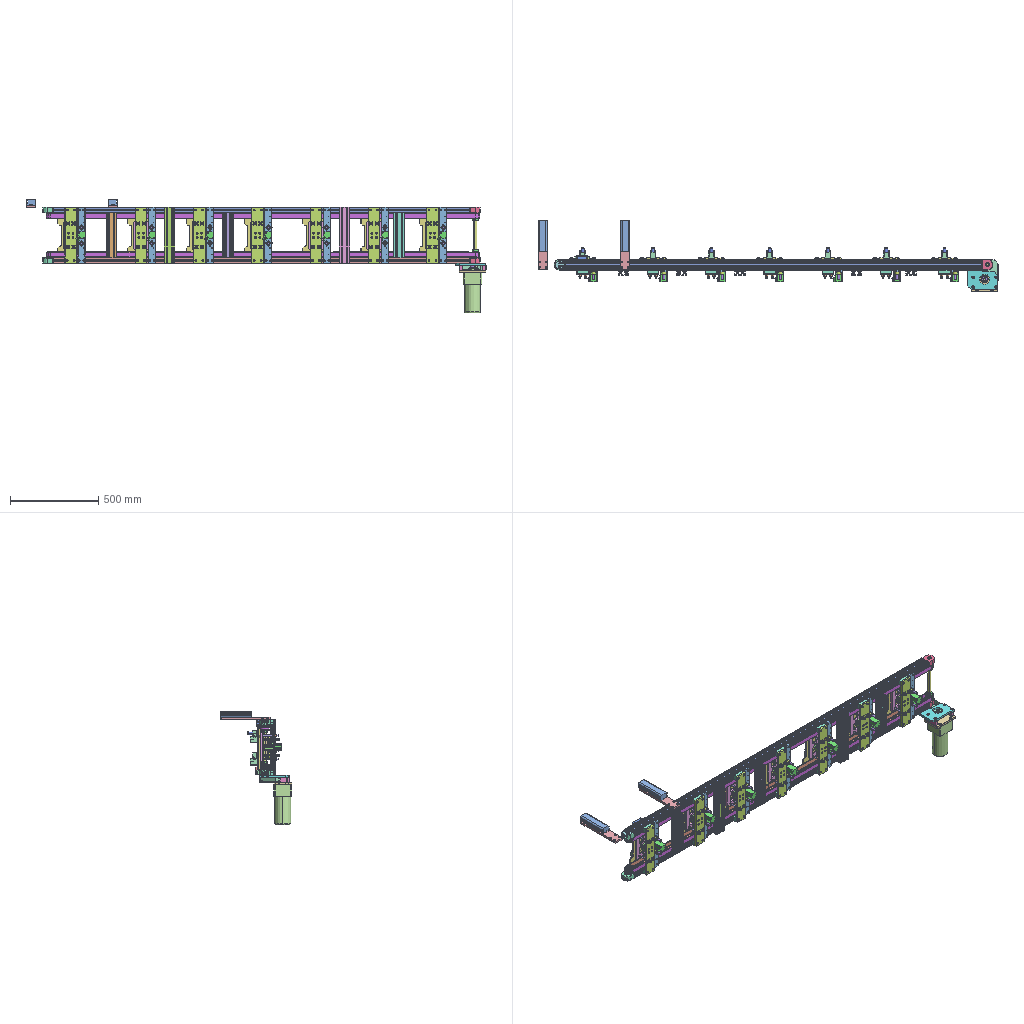Assembly | STEP file | 51 different items | 323 placed | box 2604 x 407 x 644 mm
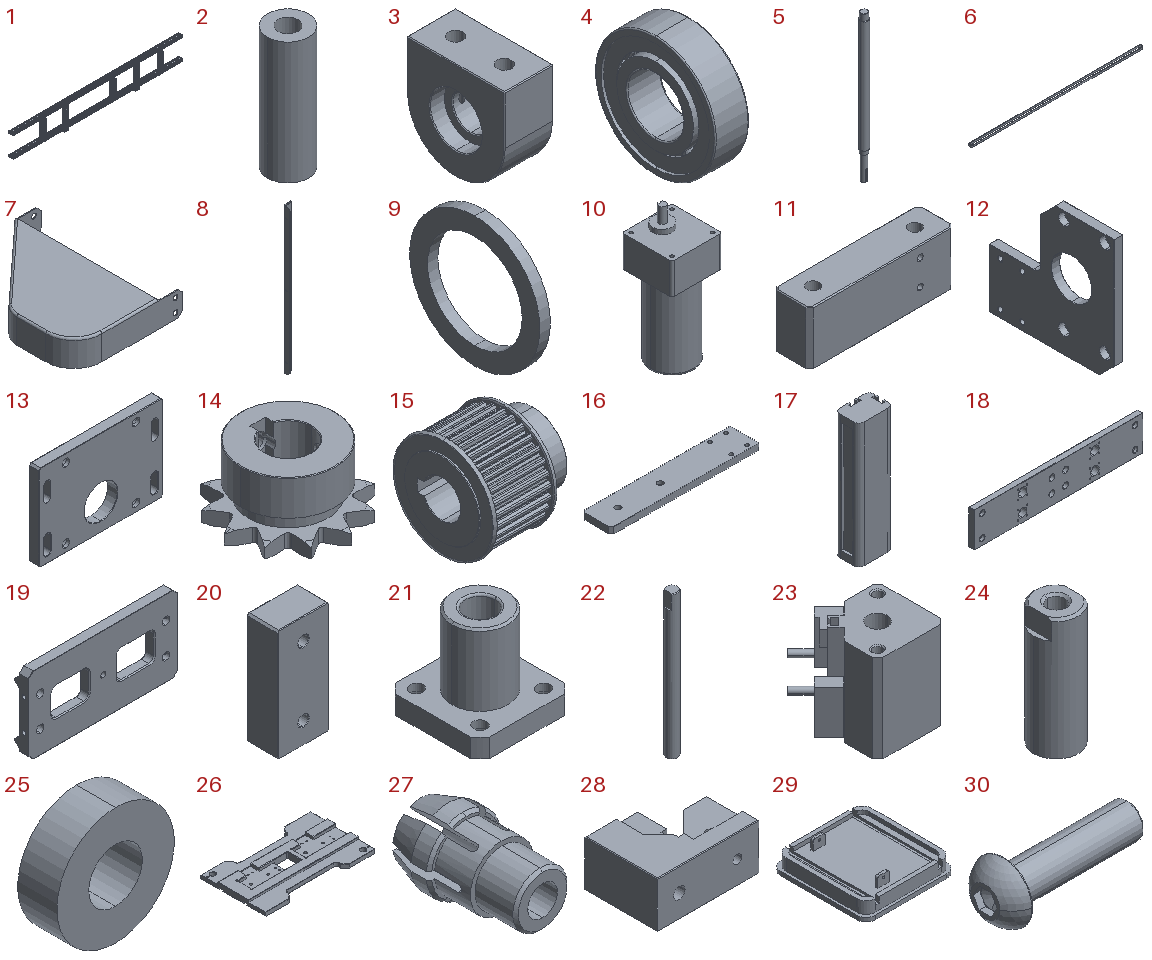Parts list (item | name | quantity | parent item | size | volume):
1 | welding conveyor bracket 01_Default <Machining> | x1 | - | 2360 x 90 x 316 mm | 3445395 mm3
2 | PN_0027 threaded bushing_Default | x8 | - | 10 x 10 x 30 mm | 1767 mm3
3 | PN_0009 hoist driving shaft fixing plate_Default | x2 | - | 30 x 60 x 60 mm | 72459 mm3
4 | GB/T 276-94 deep groove ball bearing 6002-2Z | x2 | - | 9 x 32 x 32 mm | 3545 mm3
5 | PN_0011 drive shaft_Default | x1 | - | 18 x 18 x 335 mm | 73475 mm3
6 | welding conveyor belt_Default | x2 | - | 2454 x 51.95 x 25 mm | 495464 mm3
7 | PN_0003 stopper | x1 | - | 117 x 152.64 x 28 mm | 18137 mm3
8 | PN_0005 long bracket plate_Default | x6 | - | 35 x 30 x 774.978 mm | 94609 mm3
9 | PN_0010 positioning ring_Default | x2 | - | 2 x 25 x 25 mm | 461.437 mm3
10 | Taibang reversible motor 90W_Default | x1 | in motor assembly_Default | 104 x 104 x 269 mm | 1739193 mm3
11 | PN_0002 motor pillar_Default | x2 | in motor assembly_Default | 80 x 20 x 30 mm | 45190 mm3
12 | PN_0001 motor fixing plate_Default | x1 | in motor assembly_Default | 12 x 170 x 170 mm | 228176 mm3
13 | 180W motor mounting plate_Default | x1 | in motor assembly_Default | 150 x 12 x 104 mm | 156125 mm3
14 | SP35B12_N_15_SP35B12-N-15 | x1 | in motor assembly_Default | 41 x 41 x 20 mm | 10343 mm3
15 | PN_0012 T5 synchronous pulley 30 teeth 1 | x2 | - | 44 x 49 x 49 mm | 49129 mm3
16 | PN_0004 light curtain mounting bracket plate_Default | x2 | - | 280 x 55 x 12 mm | 179701 mm3
17 | light curtain sensor_Default | x2 | - | 50 x 35 x 180 mm | 266071 mm3
18 | lifting air cylinder fixing support seat 01 | x7 | in fixture lifting mechanism assembly drawing | 316 x 10 x 65 mm | 191391 mm3
19 | lifting air cylinder fixing support seat 02 | x7 | in fixture lifting mechanism assembly drawing | 160 x 15 x 82 mm | 115095 mm3
20 | lifting air cylinder fixing support seat 03 | x14 | in fixture lifting mechanism assembly drawing | 30 x 18 x 65 mm | 34026 mm3
21 | linear bearing LMK8UU_Default | x28 | in fixture lifting mechanism assembly drawing | 25 x 25 x 24 mm | 4786 mm3
22 | positioning guide rod | x28 | in fixture lifting mechanism assembly drawing | 8 x 8 x 100 mm | 4985 mm3
23 | CDQ2A20_15D_F7NV0 | x7 | in fixture lifting mechanism assembly drawing | 48.335 x 48.335 x 46.5 mm | 53480 mm3
24 | CDQ2A20_15D_1_F7NV0 | x7 | in fixture lifting mechanism assembly drawing | 10 x 10 x 27.5 mm | 2020 mm3
25 | PN_0026 lifting mechanism plate_Default | x7 | in fixture lifting mechanism assembly drawing | 12 x 4 x 12 mm | 357.356 mm3
26 | base hole locating fixture plate | x7 | in experiment use | 255 x 150 x 14 mm | 299894 mm3
27 | 8mm elastic locating pin | x14 | in experiment use | 8.161 x 13.5 x 8.2 mm | 235.099 mm3
28 | product fixture | x28 | in product fixture_Default, experiment use | 70 x 50 x 32 mm | 81575 mm3
29 | product_Default | x12 | in product fixture_Default | 23 x 24 x 5.6 mm | 1586 mm3
30 | socket button head screw_iso_PreviewCfg | x7 | in experiment use | 68.8 x 28 x 28 mm | 15482 mm3
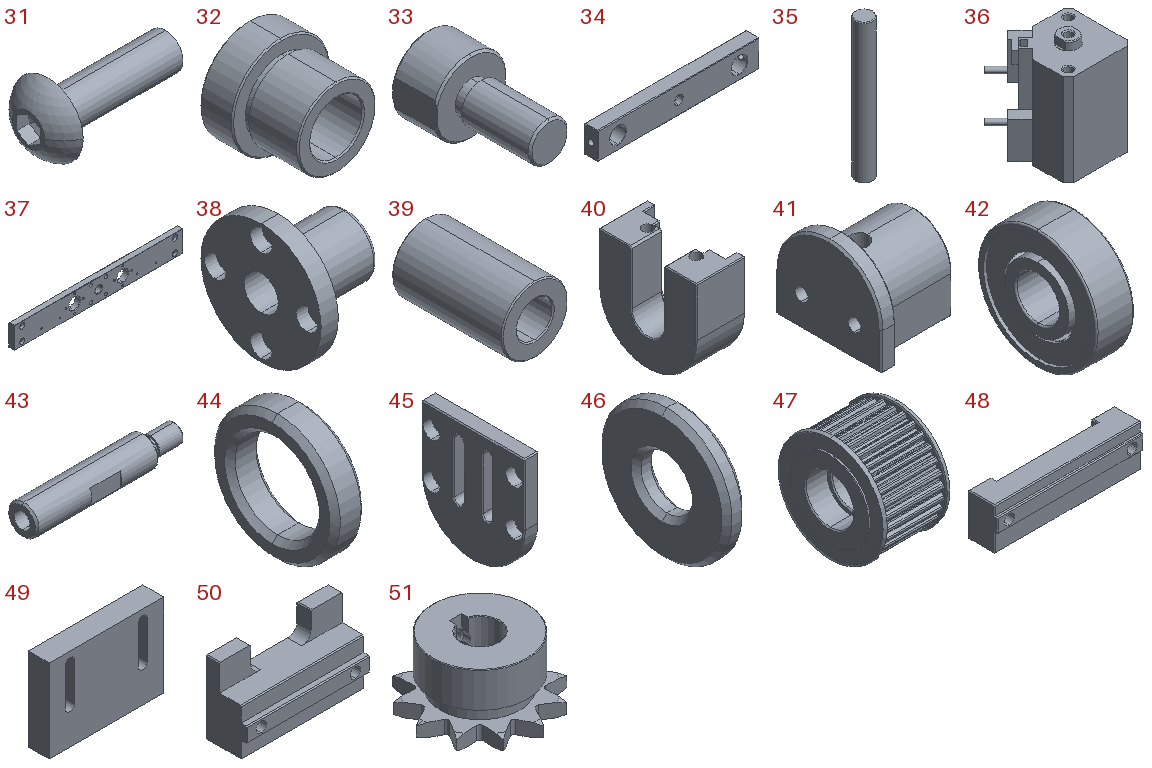31 | hexagon socket button head screws gb_PreviewCfg | x7 | in experiment use | 23.3 x 12 x 12 mm | 775.96 mm3
32 | PN_0020 side positioning guide sleeve_Default | x14 | in experiment use | 15 x 13.5 x 15 mm | 1145 mm3
33 | PN_0021 fixture block | x14 | in experiment use | 7 x 12.5 x 7.5 mm | 290.271 mm3
34 | PN_0023 lifting connecting plate_Default | x7 | in universal test stopper 12_Default | 120 x 10 x 20 mm | 20677 mm3
35 | PN_0024 test guide rod_Default | x14 | in universal test stopper 12_Default | 12 x 12 x 95 mm | 10735 mm3
36 | A_CDQ2A25-25D-F7NV012_Default | x7 | in universal test stopper 12_Default | 52.598 x 52.598 x 62.5 mm | 85379 mm3
37 | PN_0022 stopper air cylinder fixing seat | x7 | in universal test stopper 12_Default | 316 x 10 x 40 mm | 112914 mm3
38 | LHFR122_Default | x14 | in universal test stopper 12_Default | 30 x 42 x 42 mm | 12352 mm3
39 | PN_0025 lifting air cylinder extension rod_Default | x7 | in universal test stopper 12_Default | 12 x 20 x 12 mm | 1596 mm3
40 | PN_0013 driven wheel mounting plate_Default | x2 | in driven wheel assembly_Default | 30 x 60 x 60 mm | 50936 mm3
41 | PN_0014 driven wheel fixing block_Default | x2 | in driven wheel assembly_Default | 23 x 28 x 24 mm | 8364 mm3
42 | GB/T 276-94 deep groove ball bearing 608-2Z | x4 | in driven wheel assembly_Default | 7 x 22 x 22 mm | 1460 mm3
43 | PN_0016 fixed shaft_Default | x2 | in driven wheel assembly_Default | 40.5 x 8 x 8 mm | 1575 mm3
44 | PN_0017 driven wheel limiting round block_Default | x2 | in driven wheel assembly_Default | 3 x 12 x 12 mm | 168.916 mm3
45 | PN_0015 press block_Default | x2 | in driven wheel assembly_Default | 7 x 50 x 55 mm | 14443 mm3
46 | PN_0018 driven wheel fixing round block_Default | x2 | in driven wheel assembly_Default | 2 x 13 x 13 mm | 208.696 mm3
47 | PN_0019 T5 synchronous pulley 30 teeth 2 | x2 | in driven wheel assembly_Default | 32 x 49 x 49 mm | 40684 mm3
48 | PN_0006 fixture positioning -V-shape edge 2-2_Default | x1 | in press product locating assembly_Default | 80 x 16 x 23 mm | 22056 mm3
49 | PN_0007 fixture positioning -V-shape edge 1-2_Default | x1 | in press product locating assembly_Default | 55 x 10 x 40 mm | 20062 mm3
50 | PN_0008 fixture positioning plate 156 stations_Default | x1 | - | 65 x 22 x 39 mm | 33983 mm3
51 | SP35B12_N_12_SP35B12-N-12 | x1 | - | 41 x 41 x 20 mm | 11740 mm3
Placements (level | parent | child | x y z in mm | rotation matrix by rows):
1 | subassembly 2 | welding conveyor bracket 01_Default <Machining> | -0.0 -0.0 -0.0 | -1 0 0 0 1 0 0 0 -1
1 | subassembly 2 | PN_0027 threaded bushing_Default | 1150.0 15.0 -143.0 | 0 0 1 0 1 0 -1 0 0
1 | subassembly 2 | PN_0027 threaded bushing_Default | 1150.0 -15.0 -143.0 | 0 0 1 0.9242 -0.3818 0 0.3818 0.9242 0
1 | subassembly 2 | PN_0027 threaded bushing_Default | -1180.0 -15.0 143.0 | 0 0 1 0.007845 1 0 -1 0.007845 0
1 | subassembly 2 | PN_0027 threaded bushing_Default | -1180.0 15.0 143.0 | 0 0 1 0 1 0 -1 0 0
1 | subassembly 2 | PN_0027 threaded bushing_Default | -1180.0 15.0 -143.0 | 0 0 1 0 1 0 -1 0 0
1 | subassembly 2 | PN_0027 threaded bushing_Default | -1180.0 -15.0 -143.0 | 0 0 1 0 1 0 -1 0 0
1 | subassembly 2 | PN_0027 threaded bushing_Default | 1150.0 -15.0 143.0 | 0 0 1 0 1 0 -1 0 0
1 | subassembly 2 | PN_0027 threaded bushing_Default | 1150.0 15.0 143.0 | 0 0 1 0 1 0 -1 0 0
1 | subassembly 2 | PN_0009 hoist driving shaft fixing plate_Default | 1195.0 0.0 -128.0 | 0 0 -1 0 -1 0 -1 0 0
1 | subassembly 2 | PN_0009 hoist driving shaft fixing plate_Default | 1195.0 -0.0 128.0 | 0 0 -1 0 1 0 1 0 0
1 | subassembly 2 | GB/T 276-94 deep groove ball bearing 6002-2Z | 1210.0 0.0 132.5 | 0 0 -1 0 1 0 1 0 0
1 | subassembly 2 | GB/T 276-94 deep groove ball bearing 6002-2Z | 1210.0 0.0 -132.5 | 0 0 -1 0 1 0 1 0 0
1 | subassembly 2 | PN_0011 drive shaft_Default | 1210.0 -0.0 142.0 | 0.4483 -0.8939 0 0.8939 0.4483 0 0 0 1
1 | subassembly 2 | welding conveyor belt_Default | 1210.0 -0.0 -97.5 | -1 0 0 0 -1 0 0 0 1
1 | subassembly 2 | welding conveyor belt_Default | 1210.0 -0.0 122.5 | -1 0 0 0 -1 0 0 0 1
1 | subassembly 2 | PN_0003 stopper | 1241.0 -0.0 -170.0 | 0 -1 0 -1 0 0 0 0 -1
1 | subassembly 2 | PN_0005 long bracket plate_Default | -782.5 21.975 -110.5 | 0 0 -1 0 1 0 1 0 0
1 | subassembly 2 | PN_0010 positioning ring_Default | 1210.0 -0.0 -126.0 | 0 -0.5087 -0.8609 0 -0.8609 0.5087 -1 0 0
1 | subassembly 2 | PN_0010 positioning ring_Default | 1210.0 -0.0 128.0 | 0 0 1 0 1 0 -1 0 -0
1 | subassembly 2 | motor assembly_Default | 1161.778 -91.728 -283.549 | 1 0 0 0 1 0 0 0 1
2 | motor assembly_Default | Taibang reversible motor 90W_Default | 33.222 -10.273 6.549 | 1 0 0 0 1 0 0 0 1
2 | motor assembly_Default | PN_0002 motor pillar_Default | 98.222 -8.273 98.549 | 0 -1 0 1 0 0 0 0 1
2 | motor assembly_Default | PN_0002 motor pillar_Default | -31.778 -8.273 98.549 | 0 -1 0 1 0 0 0 0 1
2 | motor assembly_Default | PN_0001 motor fixing plate_Default | 23.222 36.727 125.549 | 0 0 1 0 1 0 -1 0 0
2 | motor assembly_Default | 180W motor mounting plate_Default | 33.222 -10.273 71.549 | 1 0 0 0 0 -1 0 1 0
2 | motor assembly_Default | SP35B12_N_15_SP35B12-N-15 | 33.222 9.727 93.549 | 1 0 0 0 1 0 0 0 1
1 | subassembly 2 | PN_0012 T5 synchronous pulley 30 teeth 1 | 1210.0 -0.0 -126.0 | 0 -0.8939 -0.4483 0 0.4483 -0.8939 1 0 -0
1 | subassembly 2 | PN_0012 T5 synchronous pulley 30 teeth 1 | 1210.0 -0.0 126.0 | 0 -0.8939 0.4483 0 0.4483 0.8939 -1 0 0
1 | subassembly 2 | PN_0004 light curtain mounting bracket plate_Default | -1305.745 110.0 170.0 | 0 -1 0 -1 0 0 0 0 -1
1 | subassembly 2 | light curtain sensor_Default | -1305.745 252.622 187.5 | -1 0 0 0 0 -1 0 -1 0
1 | subassembly 2 | PN_0004 light curtain mounting bracket plate_Default | -840.5 110.0 170.0 | 0 -1 0 -1 0 0 0 0 -1
1 | subassembly 2 | light curtain sensor_Default | -840.5 72.622 187.5 | 1 0 0 0 0 1 0 -1 -0
1 | subassembly 2 | PN_0005 long bracket plate_Default | 2.5 21.975 -110.5 | 0 0 -1 0 1 0 1 0 0
1 | subassembly 2 | PN_0005 long bracket plate_Default | 787.5 21.975 -110.5 | 0 0 -1 0 1 0 1 0 0
1 | subassembly 2 | PN_0005 long bracket plate_Default | 787.5 21.975 110.5 | 0 0 1 0 1 0 -1 0 0
1 | subassembly 2 | PN_0005 long bracket plate_Default | 2.5 21.975 110.5 | 0 0 1 0 1 0 -1 0 0
1 | subassembly 2 | PN_0005 long bracket plate_Default | -782.5 21.975 110.5 | 0 0 1 0 1 0 -1 0 0
1 | subassembly 2 | fixture lifting mechanism assembly drawing | -1080.0 -58.0 -0.0 | 0 0 1 0 1 0 -1 0 0
2 | fixture lifting mechanism assembly drawing | lifting air cylinder fixing support seat 01 | -0.0 -0.0 -0.0 | 1 0 0 0 1 0 0 0 1
2 | fixture lifting mechanism assembly drawing | lifting air cylinder fixing support seat 02 | -0.0 77.202 -0.0 | -1 0 0 0 1 0 0 0 -1
2 | fixture lifting mechanism assembly drawing | lifting air cylinder fixing support seat 03 | -143.0 10.0 -0.0 | 1 0 0 0 1 0 0 0 1
2 | fixture lifting mechanism assembly drawing | lifting air cylinder fixing support seat 03 | 143.0 10.0 -0.0 | -1 0 0 0 1 0 0 0 -1
2 | fixture lifting mechanism assembly drawing | linear bearing LMK8UU_Default | -67.5 15.0 -16.5 | 1 0 0 0 0 -1 0 1 -0
2 | fixture lifting mechanism assembly drawing | linear bearing LMK8UU_Default | -67.5 15.0 16.5 | 1 0 0 0 0 -1 0 1 -0
2 | fixture lifting mechanism assembly drawing | linear bearing LMK8UU_Default | 67.5 15.0 16.5 | 1 0 0 0 0 -1 0 1 -0
2 | fixture lifting mechanism assembly drawing | linear bearing LMK8UU_Default | 67.5 15.0 -16.5 | 1 0 0 0 0 -1 0 1 -0
2 | fixture lifting mechanism assembly drawing | positioning guide rod | -67.5 32.202 16.5 | 1 0 0 0 0 1 0 -1 -0
2 | fixture lifting mechanism assembly drawing | positioning guide rod | 67.5 32.202 16.5 | -1 0 0 0 0 1 0 1 0
2 | fixture lifting mechanism assembly drawing | positioning guide rod | -67.5 32.202 -16.5 | 1 0 0 0 0 1 0 -1 -0
2 | fixture lifting mechanism assembly drawing | positioning guide rod | 67.5 32.202 -16.5 | -1 0 0 0 0 1 0 1 0
2 | fixture lifting mechanism assembly drawing | CDQ2A20_15D_F7NV0 | -0.0 56.5 0.0 | 1 0 0 0 0 1 0 -1 0
2 | fixture lifting mechanism assembly drawing | CDQ2A20_15D_1_F7NV0 | -0.0 63.702 0.0 | -0.9915 0.13 0 0 0 1 0.13 0.9915 0
2 | fixture lifting mechanism assembly drawing | PN_0026 lifting mechanism plate_Default | -0.0 68.202 0.0 | 1 0 0 0 1 0 0 0 1
1 | subassembly 2 | fixture lifting mechanism assembly drawing | -682.044 -58.0 -0.0 | 0 0 1 0 1 0 -1 0 0
2 | fixture lifting mechanism assembly drawing | lifting air cylinder fixing support seat 01 | -0.0 -0.0 -0.0 | 1 0 0 0 1 0 0 0 1
2 | fixture lifting mechanism assembly drawing | lifting air cylinder fixing support seat 02 | -0.0 77.202 -0.0 | -1 0 0 0 1 0 0 0 -1
2 | fixture lifting mechanism assembly drawing | lifting air cylinder fixing support seat 03 | -143.0 10.0 -0.0 | 1 0 0 0 1 0 0 0 1
2 | fixture lifting mechanism assembly drawing | lifting air cylinder fixing support seat 03 | 143.0 10.0 -0.0 | -1 0 0 0 1 0 0 0 -1
2 | fixture lifting mechanism assembly drawing | linear bearing LMK8UU_Default | -67.5 15.0 -16.5 | 1 0 0 0 0 -1 0 1 -0
2 | fixture lifting mechanism assembly drawing | linear bearing LMK8UU_Default | -67.5 15.0 16.5 | 1 0 0 0 0 -1 0 1 -0
2 | fixture lifting mechanism assembly drawing | linear bearing LMK8UU_Default | 67.5 15.0 16.5 | 1 0 0 0 0 -1 0 1 -0
2 | fixture lifting mechanism assembly drawing | linear bearing LMK8UU_Default | 67.5 15.0 -16.5 | 1 0 0 0 0 -1 0 1 -0
2 | fixture lifting mechanism assembly drawing | positioning guide rod | -67.5 32.202 16.5 | 1 0 0 0 0 1 0 -1 -0
2 | fixture lifting mechanism assembly drawing | positioning guide rod | 67.5 32.202 16.5 | -1 0 0 0 0 1 0 1 0
2 | fixture lifting mechanism assembly drawing | positioning guide rod | -67.5 32.202 -16.5 | 1 0 0 0 0 1 0 -1 -0
2 | fixture lifting mechanism assembly drawing | positioning guide rod | 67.5 32.202 -16.5 | -1 0 0 0 0 1 0 1 0
2 | fixture lifting mechanism assembly drawing | CDQ2A20_15D_F7NV0 | -0.0 56.5 0.0 | 1 0 0 0 0 1 0 -1 0
2 | fixture lifting mechanism assembly drawing | CDQ2A20_15D_1_F7NV0 | -0.0 63.702 0.0 | -0.9915 0.13 0 0 0 1 0.13 0.9915 0
2 | fixture lifting mechanism assembly drawing | PN_0026 lifting mechanism plate_Default | -0.0 68.202 0.0 | 1 0 0 0 1 0 0 0 1
1 | subassembly 2 | experiment use | -1087.0 25.975 6.807 | 0 0 -1 0 1 0 1 0 -0
2 | experiment use | base hole locating fixture plate | -9.307 -0.0 -7.0 | 1 0 0 0 0 1 0 -1 -0
2 | experiment use | 8mm elastic locating pin | -92.307 2.5 -7.0 | 1 0 -0.006215 0 1 0 0.006215 0 1
2 | experiment use | 8mm elastic locating pin | 33.693 2.5 -7.0 | 1 0 0 0 1 0 0 0 1
2 | experiment use | product fixture_Default | -90.399 12.134 -29.041 | 1 0 0 0 1 0 0 0 1
3 | product fixture_Default | product fixture | -16.908 -5.134 22.041 | 1 0 0 0 1 0 0 0 1
3 | product fixture_Default | product_Default | 27.224 21.108 22.041 | -0.7071 0 -0.7071 -0.7071 0 0.7071 0 1 -0
2 | experiment use | product fixture_Default | 35.601 12.134 -29.041 | 1 0 0 0 1 0 0 0 1
3 | product fixture_Default | product fixture | -16.908 -5.134 22.041 | 1 0 0 0 1 0 0 0 1
3 | product fixture_Default | product_Default | 27.224 21.108 22.041 | -0.7071 0 -0.7071 -0.7071 0 0.7071 0 1 -0
2 | experiment use | socket button head screw_iso_PreviewCfg | 73.693 0.35 -7.0 | 0 -1 0 1 0 0 0 0 1
2 | experiment use | hexagon socket button head screws gb_PreviewCfg | 33.693 -0.8 -7.0 | 0 -1 0 1 0 0 0 0 1
2 | experiment use | product fixture | -107.307 7.0 -7.0 | 1 0 0 0 1 0 0 0 1
2 | experiment use | product fixture | 18.693 7.0 -7.0 | 1 0 0 0 1 0 0 0 1
2 | experiment use | PN_0020 side positioning guide sleeve_Default | 104.693 0.5 55.75 | -0.6791 0 0.734 0 1 0 -0.734 0 -0.6791
2 | experiment use | PN_0020 side positioning guide sleeve_Default | -118.307 0.5 -69.75 | 0.6258 0 -0.78 0 1 0 0.78 0 0.6258
2 | experiment use | PN_0021 fixture block | 116.193 9.0 55.75 | 1 0 0 0 1 0 0 0 1
2 | experiment use | PN_0021 fixture block | -129.807 9.0 -69.75 | 1 0 0 0 1 0 0 0 1
1 | subassembly 2 | experiment use | -689.044 25.975 6.807 | 0 0 -1 0 1 0 1 0 -0
2 | experiment use | base hole locating fixture plate | -9.307 -0.0 -7.0 | 1 0 0 0 0 1 0 -1 -0
2 | experiment use | 8mm elastic locating pin | -92.307 2.5 -7.0 | 1 0 -0.006215 0 1 0 0.006215 0 1
2 | experiment use | 8mm elastic locating pin | 33.693 2.5 -7.0 | 1 0 0 0 1 0 0 0 1
2 | experiment use | product fixture_Default | -90.399 12.134 -29.041 | 1 0 0 0 1 0 0 0 1
3 | product fixture_Default | product fixture | -16.908 -5.134 22.041 | 1 0 0 0 1 0 0 0 1
3 | product fixture_Default | product_Default | 27.224 21.108 22.041 | -0.7071 0 -0.7071 -0.7071 0 0.7071 0 1 -0
2 | experiment use | product fixture_Default | 35.601 12.134 -29.041 | 1 0 0 0 1 0 0 0 1
3 | product fixture_Default | product fixture | -16.908 -5.134 22.041 | 1 0 0 0 1 0 0 0 1
3 | product fixture_Default | product_Default | 27.224 21.108 22.041 | -0.7071 0 -0.7071 -0.7071 0 0.7071 0 1 -0
2 | experiment use | socket button head screw_iso_PreviewCfg | 73.693 0.35 -7.0 | 0 -1 0 1 0 0 0 0 1
2 | experiment use | hexagon socket button head screws gb_PreviewCfg | 33.693 -0.8 -7.0 | 0 -1 0 1 0 0 0 0 1
2 | experiment use | product fixture | -107.307 7.0 -7.0 | 1 0 0 0 1 0 0 0 1
2 | experiment use | product fixture | 18.693 7.0 -7.0 | 1 0 0 0 1 0 0 0 1
2 | experiment use | PN_0020 side positioning guide sleeve_Default | 104.693 0.5 55.75 | -0.6791 0 0.734 0 1 0 -0.734 0 -0.6791
2 | experiment use | PN_0020 side positioning guide sleeve_Default | -118.307 0.5 -69.75 | 0.6258 0 -0.78 0 1 0 0.78 0 0.6258
2 | experiment use | PN_0021 fixture block | 116.193 9.0 55.75 | 1 0 0 0 1 0 0 0 1
2 | experiment use | PN_0021 fixture block | -129.807 9.0 -69.75 | 1 0 0 0 1 0 0 0 1
1 | subassembly 2 | universal test stopper 12_Default | -1020.75 19.522 -1.088 | 0 0 -1 0 1 0 1 0 -0
2 | universal test stopper 12_Default | PN_0023 lifting connecting plate_Default | 1.088 -34.522 -1.75 | 1 0 0 0 1 0 0 0 1
2 | universal test stopper 12_Default | PN_0024 test guide rod_Default | 46.088 -7.522 -1.75 | -0.03222 -0.9995 0 0 0 -1 0.9995 -0.03222 0
2 | universal test stopper 12_Default | PN_0024 test guide rod_Default | -43.912 -7.522 -1.75 | -0.1831 -0.9831 0 0 0 -1 0.9831 -0.1831 0
2 | universal test stopper 12_Default | A_CDQ2A25-25D-F7NV012_Default | 1.088 -59.522 -1.75 | -0.008539 -1 0 0 0 1 -1 0.008539 -0
2 | universal test stopper 12_Default | PN_0022 stopper air cylinder fixing seat | 1.088 -59.522 -1.75 | 1 0 0 0 1 0 0 0 1
2 | universal test stopper 12_Default | LHFR122_Default | 46.088 -43.522 -1.75 | 0 1 0 -1 0 0 0 0 1
2 | universal test stopper 12_Default | LHFR122_Default | -43.912 -43.522 -1.75 | 0 0 -1 -1 0 0 0 1 0
2 | universal test stopper 12_Default | PN_0025 lifting air cylinder extension rod_Default | 1.088 -54.522 -1.75 | 1 0 0 0 1 0 0 0 1
1 | subassembly 2 | universal test stopper 12_Default | -622.793 19.522 -1.088 | 0 0 -1 0 1 0 1 0 -0
2 | universal test stopper 12_Default | PN_0023 lifting connecting plate_Default | 1.088 -34.522 -1.75 | 1 0 0 0 1 0 0 0 1
2 | universal test stopper 12_Default | PN_0024 test guide rod_Default | 46.088 -7.522 -1.75 | -0.03222 -0.9995 0 0 0 -1 0.9995 -0.03222 0
2 | universal test stopper 12_Default | PN_0024 test guide rod_Default | -43.912 -7.522 -1.75 | -0.1831 -0.9831 0 0 0 -1 0.9831 -0.1831 0
2 | universal test stopper 12_Default | A_CDQ2A25-25D-F7NV012_Default | 1.088 -59.522 -1.75 | -0.008539 -1 0 0 0 1 -1 0.008539 -0
2 | universal test stopper 12_Default | PN_0022 stopper air cylinder fixing seat | 1.088 -59.522 -1.75 | 1 0 0 0 1 0 0 0 1
2 | universal test stopper 12_Default | LHFR122_Default | 46.088 -43.522 -1.75 | 0 1 0 -1 0 0 0 0 1
2 | universal test stopper 12_Default | LHFR122_Default | -43.912 -43.522 -1.75 | 0 0 -1 -1 0 0 0 1 0
2 | universal test stopper 12_Default | PN_0025 lifting air cylinder extension rod_Default | 1.088 -54.522 -1.75 | 1 0 0 0 1 0 0 0 1
1 | subassembly 2 | experiment use | -359.044 25.975 6.807 | 0 0 -1 0 1 0 1 0 -0
2 | experiment use | base hole locating fixture plate | -9.307 -0.0 -7.0 | 1 0 0 0 0 1 0 -1 -0
2 | experiment use | 8mm elastic locating pin | -92.307 2.5 -7.0 | 1 0 -0.006215 0 1 0 0.006215 0 1
2 | experiment use | 8mm elastic locating pin | 33.693 2.5 -7.0 | 1 0 0 0 1 0 0 0 1
2 | experiment use | product fixture_Default | -90.399 12.134 -29.041 | 1 0 0 0 1 0 0 0 1
3 | product fixture_Default | product fixture | -16.908 -5.134 22.041 | 1 0 0 0 1 0 0 0 1
3 | product fixture_Default | product_Default | 27.224 21.108 22.041 | -0.7071 0 -0.7071 -0.7071 0 0.7071 0 1 -0
2 | experiment use | product fixture_Default | 35.601 12.134 -29.041 | 1 0 0 0 1 0 0 0 1
3 | product fixture_Default | product fixture | -16.908 -5.134 22.041 | 1 0 0 0 1 0 0 0 1
3 | product fixture_Default | product_Default | 27.224 21.108 22.041 | -0.7071 0 -0.7071 -0.7071 0 0.7071 0 1 -0
2 | experiment use | socket button head screw_iso_PreviewCfg | 73.693 0.35 -7.0 | 0 -1 0 1 0 0 0 0 1
2 | experiment use | hexagon socket button head screws gb_PreviewCfg | 33.693 -0.8 -7.0 | 0 -1 0 1 0 0 0 0 1
2 | experiment use | product fixture | -107.307 7.0 -7.0 | 1 0 0 0 1 0 0 0 1
2 | experiment use | product fixture | 18.693 7.0 -7.0 | 1 0 0 0 1 0 0 0 1
2 | experiment use | PN_0020 side positioning guide sleeve_Default | 104.693 0.5 55.75 | -0.6791 0 0.734 0 1 0 -0.734 0 -0.6791
2 | experiment use | PN_0020 side positioning guide sleeve_Default | -118.307 0.5 -69.75 | 0.6258 0 -0.78 0 1 0 0.78 0 0.6258
2 | experiment use | PN_0021 fixture block | 116.193 9.0 55.75 | 1 0 0 0 1 0 0 0 1
2 | experiment use | PN_0021 fixture block | -129.807 9.0 -69.75 | 1 0 0 0 1 0 0 0 1
1 | subassembly 2 | experiment use | -29.044 25.975 6.807 | 0 0 -1 0 1 0 1 0 -0
2 | experiment use | base hole locating fixture plate | -9.307 -0.0 -7.0 | 1 0 0 0 0 1 0 -1 -0
2 | experiment use | 8mm elastic locating pin | -92.307 2.5 -7.0 | 1 0 -0.006215 0 1 0 0.006215 0 1
2 | experiment use | 8mm elastic locating pin | 33.693 2.5 -7.0 | 1 0 0 0 1 0 0 0 1
2 | experiment use | product fixture_Default | -90.399 12.134 -29.041 | 1 0 0 0 1 0 0 0 1
3 | product fixture_Default | product fixture | -16.908 -5.134 22.041 | 1 0 0 0 1 0 0 0 1
3 | product fixture_Default | product_Default | 27.224 21.108 22.041 | -0.7071 0 -0.7071 -0.7071 0 0.7071 0 1 -0
2 | experiment use | product fixture_Default | 35.601 12.134 -29.041 | 1 0 0 0 1 0 0 0 1
3 | product fixture_Default | product fixture | -16.908 -5.134 22.041 | 1 0 0 0 1 0 0 0 1
3 | product fixture_Default | product_Default | 27.224 21.108 22.041 | -0.7071 0 -0.7071 -0.7071 0 0.7071 0 1 -0
2 | experiment use | socket button head screw_iso_PreviewCfg | 73.693 0.35 -7.0 | 0 -1 0 1 0 0 0 0 1
2 | experiment use | hexagon socket button head screws gb_PreviewCfg | 33.693 -0.8 -7.0 | 0 -1 0 1 0 0 0 0 1
2 | experiment use | product fixture | -107.307 7.0 -7.0 | 1 0 0 0 1 0 0 0 1
2 | experiment use | product fixture | 18.693 7.0 -7.0 | 1 0 0 0 1 0 0 0 1
2 | experiment use | PN_0020 side positioning guide sleeve_Default | 104.693 0.5 55.75 | -0.6791 0 0.734 0 1 0 -0.734 0 -0.6791
2 | experiment use | PN_0020 side positioning guide sleeve_Default | -118.307 0.5 -69.75 | 0.6258 0 -0.78 0 1 0 0.78 0 0.6258
2 | experiment use | PN_0021 fixture block | 116.193 9.0 55.75 | 1 0 0 0 1 0 0 0 1
2 | experiment use | PN_0021 fixture block | -129.807 9.0 -69.75 | 1 0 0 0 1 0 0 0 1
1 | subassembly 2 | experiment use | 300.956 25.975 6.807 | 0 0 -1 0 1 0 1 0 -0
2 | experiment use | base hole locating fixture plate | -9.307 -0.0 -7.0 | 1 0 0 0 0 1 0 -1 -0
2 | experiment use | 8mm elastic locating pin | -92.307 2.5 -7.0 | 1 0 -0.006215 0 1 0 0.006215 0 1
2 | experiment use | 8mm elastic locating pin | 33.693 2.5 -7.0 | 1 0 0 0 1 0 0 0 1
2 | experiment use | product fixture_Default | -90.399 12.134 -29.041 | 1 0 0 0 1 0 0 0 1
3 | product fixture_Default | product fixture | -16.908 -5.134 22.041 | 1 0 0 0 1 0 0 0 1
2 | experiment use | product fixture_Default | 35.601 12.134 -29.041 | 1 0 0 0 1 0 0 0 1
3 | product fixture_Default | product fixture | -16.908 -5.134 22.041 | 1 0 0 0 1 0 0 0 1
2 | experiment use | socket button head screw_iso_PreviewCfg | 73.693 0.35 -7.0 | 0 -1 0 1 0 0 0 0 1
2 | experiment use | hexagon socket button head screws gb_PreviewCfg | 33.693 -0.8 -7.0 | 0 -1 0 1 0 0 0 0 1
2 | experiment use | product fixture | -107.307 7.0 -7.0 | 1 0 0 0 1 0 0 0 1
2 | experiment use | product fixture | 18.693 7.0 -7.0 | 1 0 0 0 1 0 0 0 1
2 | experiment use | PN_0020 side positioning guide sleeve_Default | 104.693 0.5 55.75 | -0.6791 0 0.734 0 1 0 -0.734 0 -0.6791
2 | experiment use | PN_0020 side positioning guide sleeve_Default | -118.307 0.5 -69.75 | 0.6258 0 -0.78 0 1 0 0.78 0 0.6258
2 | experiment use | PN_0021 fixture block | 116.193 9.0 55.75 | 1 0 0 0 1 0 0 0 1
2 | experiment use | PN_0021 fixture block | -129.807 9.0 -69.75 | 1 0 0 0 1 0 0 0 1
1 | subassembly 2 | experiment use | 630.956 25.975 6.807 | 0 0 -1 0 1 0 1 0 -0
2 | experiment use | base hole locating fixture plate | -9.307 -0.0 -7.0 | 1 0 0 0 0 1 0 -1 -0
2 | experiment use | 8mm elastic locating pin | -92.307 2.5 -7.0 | 1 0 -0.006215 0 1 0 0.006215 0 1
2 | experiment use | 8mm elastic locating pin | 33.693 2.5 -7.0 | 1 0 0 0 1 0 0 0 1
2 | experiment use | product fixture_Default | -90.399 12.134 -29.041 | 1 0 0 0 1 0 0 0 1
3 | product fixture_Default | product fixture | -16.908 -5.134 22.041 | 1 0 0 0 1 0 0 0 1
3 | product fixture_Default | product_Default | 27.224 21.108 22.041 | -0.7071 0 -0.7071 -0.7071 0 0.7071 0 1 -0
2 | experiment use | product fixture_Default | 35.601 12.134 -29.041 | 1 0 0 0 1 0 0 0 1
3 | product fixture_Default | product fixture | -16.908 -5.134 22.041 | 1 0 0 0 1 0 0 0 1
3 | product fixture_Default | product_Default | 27.224 21.108 22.041 | -0.7071 0 -0.7071 -0.7071 0 0.7071 0 1 -0
2 | experiment use | socket button head screw_iso_PreviewCfg | 73.693 0.35 -7.0 | 0 -1 0 1 0 0 0 0 1
2 | experiment use | hexagon socket button head screws gb_PreviewCfg | 33.693 -0.8 -7.0 | 0 -1 0 1 0 0 0 0 1
2 | experiment use | product fixture | -107.307 7.0 -7.0 | 1 0 0 0 1 0 0 0 1
2 | experiment use | product fixture | 18.693 7.0 -7.0 | 1 0 0 0 1 0 0 0 1
2 | experiment use | PN_0020 side positioning guide sleeve_Default | 104.693 0.5 55.75 | -0.6791 0 0.734 0 1 0 -0.734 0 -0.6791
2 | experiment use | PN_0020 side positioning guide sleeve_Default | -118.307 0.5 -69.75 | 0.6258 0 -0.78 0 1 0 0.78 0 0.6258
2 | experiment use | PN_0021 fixture block | 116.193 9.0 55.75 | 1 0 0 0 1 0 0 0 1
2 | experiment use | PN_0021 fixture block | -129.807 9.0 -69.75 | 1 0 0 0 1 0 0 0 1
1 | subassembly 2 | experiment use | 960.956 25.975 6.807 | 0 0 -1 0 1 0 1 0 -0
2 | experiment use | base hole locating fixture plate | -9.307 -0.0 -7.0 | 1 0 0 0 0 1 0 -1 -0
2 | experiment use | 8mm elastic locating pin | -92.307 2.5 -7.0 | 1 0 -0.006215 0 1 0 0.006215 0 1
2 | experiment use | 8mm elastic locating pin | 33.693 2.5 -7.0 | 1 0 0 0 1 0 0 0 1
2 | experiment use | product fixture_Default | -90.399 12.134 -29.041 | 1 0 0 0 1 0 0 0 1
3 | product fixture_Default | product fixture | -16.908 -5.134 22.041 | 1 0 0 0 1 0 0 0 1
3 | product fixture_Default | product_Default | 27.224 21.108 22.041 | -0.7071 0 -0.7071 -0.7071 0 0.7071 0 1 -0
2 | experiment use | product fixture_Default | 35.601 12.134 -29.041 | 1 0 0 0 1 0 0 0 1
3 | product fixture_Default | product fixture | -16.908 -5.134 22.041 | 1 0 0 0 1 0 0 0 1
3 | product fixture_Default | product_Default | 27.224 21.108 22.041 | -0.7071 0 -0.7071 -0.7071 0 0.7071 0 1 -0
2 | experiment use | socket button head screw_iso_PreviewCfg | 73.693 0.35 -7.0 | 0 -1 0 1 0 0 0 0 1
2 | experiment use | hexagon socket button head screws gb_PreviewCfg | 33.693 -0.8 -7.0 | 0 -1 0 1 0 0 0 0 1
2 | experiment use | product fixture | -107.307 7.0 -7.0 | 1 0 0 0 1 0 0 0 1
2 | experiment use | product fixture | 18.693 7.0 -7.0 | 1 0 0 0 1 0 0 0 1
2 | experiment use | PN_0020 side positioning guide sleeve_Default | 104.693 0.5 55.75 | -0.6791 0 0.734 0 1 0 -0.734 0 -0.6791
2 | experiment use | PN_0020 side positioning guide sleeve_Default | -118.307 0.5 -69.75 | 0.6258 0 -0.78 0 1 0 0.78 0 0.6258
2 | experiment use | PN_0021 fixture block | 116.193 9.0 55.75 | 1 0 0 0 1 0 0 0 1
2 | experiment use | PN_0021 fixture block | -129.807 9.0 -69.75 | 1 0 0 0 1 0 0 0 1
1 | subassembly 2 | fixture lifting mechanism assembly drawing | -352.044 -58.0 0.0 | 0 0 1 0 1 0 -1 0 0
2 | fixture lifting mechanism assembly drawing | lifting air cylinder fixing support seat 01 | -0.0 -0.0 -0.0 | 1 0 0 0 1 0 0 0 1
2 | fixture lifting mechanism assembly drawing | lifting air cylinder fixing support seat 02 | -0.0 77.202 -0.0 | -1 0 0 0 1 0 0 0 -1
2 | fixture lifting mechanism assembly drawing | lifting air cylinder fixing support seat 03 | -143.0 10.0 -0.0 | 1 0 0 0 1 0 0 0 1
2 | fixture lifting mechanism assembly drawing | lifting air cylinder fixing support seat 03 | 143.0 10.0 -0.0 | -1 0 0 0 1 0 0 0 -1
2 | fixture lifting mechanism assembly drawing | linear bearing LMK8UU_Default | -67.5 15.0 -16.5 | 1 0 0 0 0 -1 0 1 -0
2 | fixture lifting mechanism assembly drawing | linear bearing LMK8UU_Default | -67.5 15.0 16.5 | 1 0 0 0 0 -1 0 1 -0
2 | fixture lifting mechanism assembly drawing | linear bearing LMK8UU_Default | 67.5 15.0 16.5 | 1 0 0 0 0 -1 0 1 -0
2 | fixture lifting mechanism assembly drawing | linear bearing LMK8UU_Default | 67.5 15.0 -16.5 | 1 0 0 0 0 -1 0 1 -0
2 | fixture lifting mechanism assembly drawing | positioning guide rod | -67.5 32.202 16.5 | 1 0 0 0 0 1 0 -1 -0
2 | fixture lifting mechanism assembly drawing | positioning guide rod | 67.5 32.202 16.5 | -1 0 0 0 0 1 0 1 0
2 | fixture lifting mechanism assembly drawing | positioning guide rod | -67.5 32.202 -16.5 | 1 0 0 0 0 1 0 -1 -0
2 | fixture lifting mechanism assembly drawing | positioning guide rod | 67.5 32.202 -16.5 | -1 0 0 0 0 1 0 1 0
2 | fixture lifting mechanism assembly drawing | CDQ2A20_15D_F7NV0 | -0.0 56.5 0.0 | 1 0 0 0 0 1 0 -1 0
2 | fixture lifting mechanism assembly drawing | CDQ2A20_15D_1_F7NV0 | -0.0 63.702 0.0 | -0.9915 0.13 0 0 0 1 0.13 0.9915 0
2 | fixture lifting mechanism assembly drawing | PN_0026 lifting mechanism plate_Default | -0.0 68.202 0.0 | 1 0 0 0 1 0 0 0 1
1 | subassembly 2 | fixture lifting mechanism assembly drawing | -22.044 -58.0 0.0 | 0 0 1 0 1 0 -1 0 0
2 | fixture lifting mechanism assembly drawing | lifting air cylinder fixing support seat 01 | -0.0 -0.0 -0.0 | 1 0 0 0 1 0 0 0 1
2 | fixture lifting mechanism assembly drawing | lifting air cylinder fixing support seat 02 | -0.0 77.202 -0.0 | -1 0 0 0 1 0 0 0 -1
2 | fixture lifting mechanism assembly drawing | lifting air cylinder fixing support seat 03 | -143.0 10.0 -0.0 | 1 0 0 0 1 0 0 0 1
2 | fixture lifting mechanism assembly drawing | lifting air cylinder fixing support seat 03 | 143.0 10.0 -0.0 | -1 0 0 0 1 0 0 0 -1
2 | fixture lifting mechanism assembly drawing | linear bearing LMK8UU_Default | -67.5 15.0 -16.5 | 1 0 0 0 0 -1 0 1 -0
2 | fixture lifting mechanism assembly drawing | linear bearing LMK8UU_Default | -67.5 15.0 16.5 | 1 0 0 0 0 -1 0 1 -0
2 | fixture lifting mechanism assembly drawing | linear bearing LMK8UU_Default | 67.5 15.0 16.5 | 1 0 0 0 0 -1 0 1 -0
2 | fixture lifting mechanism assembly drawing | linear bearing LMK8UU_Default | 67.5 15.0 -16.5 | 1 0 0 0 0 -1 0 1 -0
2 | fixture lifting mechanism assembly drawing | positioning guide rod | -67.5 32.202 16.5 | 1 0 0 0 0 1 0 -1 -0
2 | fixture lifting mechanism assembly drawing | positioning guide rod | 67.5 32.202 16.5 | -1 0 0 0 0 1 0 1 0
2 | fixture lifting mechanism assembly drawing | positioning guide rod | -67.5 32.202 -16.5 | 1 0 0 0 0 1 0 -1 -0
2 | fixture lifting mechanism assembly drawing | positioning guide rod | 67.5 32.202 -16.5 | -1 0 0 0 0 1 0 1 0
2 | fixture lifting mechanism assembly drawing | CDQ2A20_15D_F7NV0 | -0.0 56.5 0.0 | 1 0 0 0 0 1 0 -1 0
2 | fixture lifting mechanism assembly drawing | CDQ2A20_15D_1_F7NV0 | -0.0 63.702 0.0 | -0.9915 0.13 0 0 0 1 0.13 0.9915 0
2 | fixture lifting mechanism assembly drawing | PN_0026 lifting mechanism plate_Default | -0.0 68.202 0.0 | 1 0 0 0 1 0 0 0 1
1 | subassembly 2 | fixture lifting mechanism assembly drawing | 307.956 -58.0 0.0 | 0 0 1 0 1 0 -1 0 0
2 | fixture lifting mechanism assembly drawing | lifting air cylinder fixing support seat 01 | -0.0 -0.0 -0.0 | 1 0 0 0 1 0 0 0 1
2 | fixture lifting mechanism assembly drawing | lifting air cylinder fixing support seat 02 | -0.0 77.202 -0.0 | -1 0 0 0 1 0 0 0 -1
2 | fixture lifting mechanism assembly drawing | lifting air cylinder fixing support seat 03 | -143.0 10.0 -0.0 | 1 0 0 0 1 0 0 0 1
2 | fixture lifting mechanism assembly drawing | lifting air cylinder fixing support seat 03 | 143.0 10.0 -0.0 | -1 0 0 0 1 0 0 0 -1
2 | fixture lifting mechanism assembly drawing | linear bearing LMK8UU_Default | -67.5 15.0 -16.5 | 1 0 0 0 0 -1 0 1 -0
2 | fixture lifting mechanism assembly drawing | linear bearing LMK8UU_Default | -67.5 15.0 16.5 | 1 0 0 0 0 -1 0 1 -0
2 | fixture lifting mechanism assembly drawing | linear bearing LMK8UU_Default | 67.5 15.0 16.5 | 1 0 0 0 0 -1 0 1 -0
2 | fixture lifting mechanism assembly drawing | linear bearing LMK8UU_Default | 67.5 15.0 -16.5 | 1 0 0 0 0 -1 0 1 -0
2 | fixture lifting mechanism assembly drawing | positioning guide rod | -67.5 32.202 16.5 | 1 0 0 0 0 1 0 -1 -0
2 | fixture lifting mechanism assembly drawing | positioning guide rod | 67.5 32.202 16.5 | -1 0 0 0 0 1 0 1 0
2 | fixture lifting mechanism assembly drawing | positioning guide rod | -67.5 32.202 -16.5 | 1 0 0 0 0 1 0 -1 -0
2 | fixture lifting mechanism assembly drawing | positioning guide rod | 67.5 32.202 -16.5 | -1 0 0 0 0 1 0 1 0
2 | fixture lifting mechanism assembly drawing | CDQ2A20_15D_F7NV0 | -0.0 56.5 0.0 | 1 0 0 0 0 1 0 -1 0
2 | fixture lifting mechanism assembly drawing | CDQ2A20_15D_1_F7NV0 | -0.0 63.702 0.0 | -0.9915 0.13 0 0 0 1 0.13 0.9915 0
2 | fixture lifting mechanism assembly drawing | PN_0026 lifting mechanism plate_Default | -0.0 68.202 0.0 | 1 0 0 0 1 0 0 0 1
1 | subassembly 2 | fixture lifting mechanism assembly drawing | 637.956 -58.0 0.0 | 0 0 1 0 1 0 -1 0 0
2 | fixture lifting mechanism assembly drawing | lifting air cylinder fixing support seat 01 | -0.0 -0.0 -0.0 | 1 0 0 0 1 0 0 0 1
2 | fixture lifting mechanism assembly drawing | lifting air cylinder fixing support seat 02 | -0.0 77.202 -0.0 | -1 0 0 0 1 0 0 0 -1
2 | fixture lifting mechanism assembly drawing | lifting air cylinder fixing support seat 03 | -143.0 10.0 -0.0 | 1 0 0 0 1 0 0 0 1
2 | fixture lifting mechanism assembly drawing | lifting air cylinder fixing support seat 03 | 143.0 10.0 -0.0 | -1 0 0 0 1 0 0 0 -1
2 | fixture lifting mechanism assembly drawing | linear bearing LMK8UU_Default | -67.5 15.0 -16.5 | 1 0 0 0 0 -1 0 1 -0
2 | fixture lifting mechanism assembly drawing | linear bearing LMK8UU_Default | -67.5 15.0 16.5 | 1 0 0 0 0 -1 0 1 -0
2 | fixture lifting mechanism assembly drawing | linear bearing LMK8UU_Default | 67.5 15.0 16.5 | 1 0 0 0 0 -1 0 1 -0
2 | fixture lifting mechanism assembly drawing | linear bearing LMK8UU_Default | 67.5 15.0 -16.5 | 1 0 0 0 0 -1 0 1 -0
2 | fixture lifting mechanism assembly drawing | positioning guide rod | -67.5 32.202 16.5 | 1 0 0 0 0 1 0 -1 -0
2 | fixture lifting mechanism assembly drawing | positioning guide rod | 67.5 32.202 16.5 | -1 0 0 0 0 1 0 1 0
2 | fixture lifting mechanism assembly drawing | positioning guide rod | -67.5 32.202 -16.5 | 1 0 0 0 0 1 0 -1 -0
2 | fixture lifting mechanism assembly drawing | positioning guide rod | 67.5 32.202 -16.5 | -1 0 0 0 0 1 0 1 0
2 | fixture lifting mechanism assembly drawing | CDQ2A20_15D_F7NV0 | -0.0 56.5 0.0 | 1 0 0 0 0 1 0 -1 0
2 | fixture lifting mechanism assembly drawing | CDQ2A20_15D_1_F7NV0 | -0.0 63.702 0.0 | -0.9915 0.13 0 0 0 1 0.13 0.9915 0
2 | fixture lifting mechanism assembly drawing | PN_0026 lifting mechanism plate_Default | -0.0 68.202 0.0 | 1 0 0 0 1 0 0 0 1
1 | subassembly 2 | fixture lifting mechanism assembly drawing | 967.956 -58.0 0.0 | 0 0 1 0 1 0 -1 0 0
2 | fixture lifting mechanism assembly drawing | lifting air cylinder fixing support seat 01 | -0.0 -0.0 -0.0 | 1 0 0 0 1 0 0 0 1
2 | fixture lifting mechanism assembly drawing | lifting air cylinder fixing support seat 02 | -0.0 77.202 -0.0 | -1 0 0 0 1 0 0 0 -1
2 | fixture lifting mechanism assembly drawing | lifting air cylinder fixing support seat 03 | -143.0 10.0 -0.0 | 1 0 0 0 1 0 0 0 1
2 | fixture lifting mechanism assembly drawing | lifting air cylinder fixing support seat 03 | 143.0 10.0 -0.0 | -1 0 0 0 1 0 0 0 -1
2 | fixture lifting mechanism assembly drawing | linear bearing LMK8UU_Default | -67.5 15.0 -16.5 | 1 0 0 0 0 -1 0 1 -0
2 | fixture lifting mechanism assembly drawing | linear bearing LMK8UU_Default | -67.5 15.0 16.5 | 1 0 0 0 0 -1 0 1 -0
2 | fixture lifting mechanism assembly drawing | linear bearing LMK8UU_Default | 67.5 15.0 16.5 | 1 0 0 0 0 -1 0 1 -0
2 | fixture lifting mechanism assembly drawing | linear bearing LMK8UU_Default | 67.5 15.0 -16.5 | 1 0 0 0 0 -1 0 1 -0
2 | fixture lifting mechanism assembly drawing | positioning guide rod | -67.5 32.202 16.5 | 1 0 0 0 0 1 0 -1 -0
2 | fixture lifting mechanism assembly drawing | positioning guide rod | 67.5 32.202 16.5 | -1 0 0 0 0 1 0 1 0
2 | fixture lifting mechanism assembly drawing | positioning guide rod | -67.5 32.202 -16.5 | 1 0 0 0 0 1 0 -1 -0
2 | fixture lifting mechanism assembly drawing | positioning guide rod | 67.5 32.202 -16.5 | -1 0 0 0 0 1 0 1 0
2 | fixture lifting mechanism assembly drawing | CDQ2A20_15D_F7NV0 | -0.0 56.5 0.0 | 1 0 0 0 0 1 0 -1 0
2 | fixture lifting mechanism assembly drawing | CDQ2A20_15D_1_F7NV0 | -0.0 63.702 0.0 | -0.9915 0.13 0 0 0 1 0.13 0.9915 0
2 | fixture lifting mechanism assembly drawing | PN_0026 lifting mechanism plate_Default | -0.0 68.202 0.0 | 1 0 0 0 1 0 0 0 1
1 | subassembly 2 | universal test stopper 12_Default | -292.793 19.522 -1.088 | 0 0 -1 0 1 0 1 0 -0
2 | universal test stopper 12_Default | PN_0023 lifting connecting plate_Default | 1.088 -34.522 -1.75 | 1 0 0 0 1 0 0 0 1
2 | universal test stopper 12_Default | PN_0024 test guide rod_Default | 46.088 -7.522 -1.75 | -0.03222 -0.9995 0 0 0 -1 0.9995 -0.03222 0
2 | universal test stopper 12_Default | PN_0024 test guide rod_Default | -43.912 -7.522 -1.75 | -0.1831 -0.9831 0 0 0 -1 0.9831 -0.1831 0
2 | universal test stopper 12_Default | A_CDQ2A25-25D-F7NV012_Default | 1.088 -59.522 -1.75 | -0.008539 -1 0 0 0 1 -1 0.008539 -0
2 | universal test stopper 12_Default | PN_0022 stopper air cylinder fixing seat | 1.088 -59.522 -1.75 | 1 0 0 0 1 0 0 0 1
2 | universal test stopper 12_Default | LHFR122_Default | 46.088 -43.522 -1.75 | 0 1 0 -1 0 0 0 0 1
2 | universal test stopper 12_Default | LHFR122_Default | -43.912 -43.522 -1.75 | 0 0 -1 -1 0 0 0 1 0
2 | universal test stopper 12_Default | PN_0025 lifting air cylinder extension rod_Default | 1.088 -54.522 -1.75 | 1 0 0 0 1 0 0 0 1
1 | subassembly 2 | universal test stopper 12_Default | 37.207 19.522 -1.088 | 0 0 -1 0 1 0 1 0 -0
2 | universal test stopper 12_Default | PN_0023 lifting connecting plate_Default | 1.088 -34.522 -1.75 | 1 0 0 0 1 0 0 0 1
2 | universal test stopper 12_Default | PN_0024 test guide rod_Default | 46.088 -7.522 -1.75 | -0.03222 -0.9995 0 0 0 -1 0.9995 -0.03222 0
2 | universal test stopper 12_Default | PN_0024 test guide rod_Default | -43.912 -7.522 -1.75 | -0.1831 -0.9831 0 0 0 -1 0.9831 -0.1831 0
2 | universal test stopper 12_Default | A_CDQ2A25-25D-F7NV012_Default | 1.088 -59.522 -1.75 | -0.008539 -1 0 0 0 1 -1 0.008539 -0
2 | universal test stopper 12_Default | PN_0022 stopper air cylinder fixing seat | 1.088 -59.522 -1.75 | 1 0 0 0 1 0 0 0 1
2 | universal test stopper 12_Default | LHFR122_Default | 46.088 -43.522 -1.75 | 0 1 0 -1 0 0 0 0 1
2 | universal test stopper 12_Default | LHFR122_Default | -43.912 -43.522 -1.75 | 0 0 -1 -1 0 0 0 1 0
2 | universal test stopper 12_Default | PN_0025 lifting air cylinder extension rod_Default | 1.088 -54.522 -1.75 | 1 0 0 0 1 0 0 0 1
1 | subassembly 2 | universal test stopper 12_Default | 367.207 19.522 -1.088 | 0 0 -1 0 1 0 1 0 -0
2 | universal test stopper 12_Default | PN_0023 lifting connecting plate_Default | 1.088 -34.522 -1.75 | 1 0 0 0 1 0 0 0 1
2 | universal test stopper 12_Default | PN_0024 test guide rod_Default | 46.088 -7.522 -1.75 | -0.03222 -0.9995 0 0 0 -1 0.9995 -0.03222 0
2 | universal test stopper 12_Default | PN_0024 test guide rod_Default | -43.912 -7.522 -1.75 | -0.1831 -0.9831 0 0 0 -1 0.9831 -0.1831 0
2 | universal test stopper 12_Default | A_CDQ2A25-25D-F7NV012_Default | 1.088 -59.522 -1.75 | -0.008539 -1 0 0 0 1 -1 0.008539 -0
2 | universal test stopper 12_Default | PN_0022 stopper air cylinder fixing seat | 1.088 -59.522 -1.75 | 1 0 0 0 1 0 0 0 1
2 | universal test stopper 12_Default | LHFR122_Default | 46.088 -43.522 -1.75 | 0 1 0 -1 0 0 0 0 1
2 | universal test stopper 12_Default | LHFR122_Default | -43.912 -43.522 -1.75 | 0 0 -1 -1 0 0 0 1 0
2 | universal test stopper 12_Default | PN_0025 lifting air cylinder extension rod_Default | 1.088 -54.522 -1.75 | 1 0 0 0 1 0 0 0 1
1 | subassembly 2 | universal test stopper 12_Default | 697.207 19.522 -1.088 | 0 0 -1 0 1 0 1 0 -0
2 | universal test stopper 12_Default | PN_0023 lifting connecting plate_Default | 1.088 -34.522 -1.75 | 1 0 0 0 1 0 0 0 1
2 | universal test stopper 12_Default | PN_0024 test guide rod_Default | 46.088 -7.522 -1.75 | -0.03222 -0.9995 0 0 0 -1 0.9995 -0.03222 0
2 | universal test stopper 12_Default | PN_0024 test guide rod_Default | -43.912 -7.522 -1.75 | -0.1831 -0.9831 0 0 0 -1 0.9831 -0.1831 0
2 | universal test stopper 12_Default | A_CDQ2A25-25D-F7NV012_Default | 1.088 -59.522 -1.75 | -0.008539 -1 0 0 0 1 -1 0.008539 -0
2 | universal test stopper 12_Default | PN_0022 stopper air cylinder fixing seat | 1.088 -59.522 -1.75 | 1 0 0 0 1 0 0 0 1
2 | universal test stopper 12_Default | LHFR122_Default | 46.088 -43.522 -1.75 | 0 1 0 -1 0 0 0 0 1
2 | universal test stopper 12_Default | LHFR122_Default | -43.912 -43.522 -1.75 | 0 0 -1 -1 0 0 0 1 0
2 | universal test stopper 12_Default | PN_0025 lifting air cylinder extension rod_Default | 1.088 -54.522 -1.75 | 1 0 0 0 1 0 0 0 1
1 | subassembly 2 | universal test stopper 12_Default | 1027.207 19.522 -1.088 | 0 0 -1 0 1 0 1 0 -0
2 | universal test stopper 12_Default | PN_0023 lifting connecting plate_Default | 1.088 -34.522 -1.75 | 1 0 0 0 1 0 0 0 1
2 | universal test stopper 12_Default | PN_0024 test guide rod_Default | 46.088 -7.522 -1.75 | -0.03222 -0.9995 0 0 0 -1 0.9995 -0.03222 0
2 | universal test stopper 12_Default | PN_0024 test guide rod_Default | -43.912 -7.522 -1.75 | -0.1831 -0.9831 0 0 0 -1 0.9831 -0.1831 0
2 | universal test stopper 12_Default | A_CDQ2A25-25D-F7NV012_Default | 1.088 -59.522 -1.75 | -0.008539 -1 0 0 0 1 -1 0.008539 -0
2 | universal test stopper 12_Default | PN_0022 stopper air cylinder fixing seat | 1.088 -59.522 -1.75 | 1 0 0 0 1 0 0 0 1
2 | universal test stopper 12_Default | LHFR122_Default | 46.088 -43.522 -1.75 | 0 1 0 -1 0 0 0 0 1
2 | universal test stopper 12_Default | LHFR122_Default | -43.912 -43.522 -1.75 | 0 0 -1 -1 0 0 0 1 0
2 | universal test stopper 12_Default | PN_0025 lifting air cylinder extension rod_Default | 1.088 -54.522 -1.75 | 1 0 0 0 1 0 0 0 1
1 | subassembly 2 | driven wheel assembly_Default | -1195.0 -0.0 -128.0 | 0 0 1 0 1 0 -1 0 -0
2 | driven wheel assembly_Default | PN_0013 driven wheel mounting plate_Default | -0.0 -0.0 -0.0 | 1 0 0 0 1 0 0 0 1
2 | driven wheel assembly_Default | PN_0014 driven wheel fixing block_Default | 23.0 0.0 15.0 | -1 0 0 0 1 0 0 0 -1
2 | driven wheel assembly_Default | GB/T 276-94 deep groove ball bearing 608-2Z | -27.5 -0.0 2.73 | 1 0 0 0 -0.000286 -1 0 1 -0.000286
2 | driven wheel assembly_Default | PN_0016 fixed shaft_Default | -32.5 0.0 2.73 | 1 0 0 0 -1 0 0 0 -1
2 | driven wheel assembly_Default | GB/T 276-94 deep groove ball bearing 608-2Z | -6.5 -0.0 2.73 | -1 0 0 0 -0.9992 0.03909 0 0.03909 0.9992
2 | driven wheel assembly_Default | PN_0017 driven wheel limiting round block_Default | 0.0 0.0 2.73 | -1 0 0 0 0.1471 -0.9891 0 -0.9891 -0.1471
2 | driven wheel assembly_Default | PN_0015 press block_Default | 30.0 -0.0 15.0 | -1 0 0 0 -1 0 0 0 1
2 | driven wheel assembly_Default | PN_0018 driven wheel fixing round block_Default | -33.0 -0.0 2.73 | 1 0 0 0 0.9757 0.2192 0 -0.2192 0.9757
2 | driven wheel assembly_Default | PN_0019 T5 synchronous pulley 30 teeth 2 | -34.0 -0.0 2.73 | 1 0 0 0 1 0 0 0 1
1 | subassembly 2 | driven wheel assembly_Default | -1195.0 -0.0 128.0 | 0 0 1 0 -1 0 1 0 -0
2 | driven wheel assembly_Default | PN_0013 driven wheel mounting plate_Default | -0.0 -0.0 -0.0 | 1 0 0 0 1 0 0 0 1
2 | driven wheel assembly_Default | PN_0014 driven wheel fixing block_Default | 23.0 0.0 15.0 | -1 0 0 0 1 0 0 0 -1
2 | driven wheel assembly_Default | GB/T 276-94 deep groove ball bearing 608-2Z | -27.5 -0.0 2.73 | 1 0 0 0 -0.000286 -1 0 1 -0.000286
2 | driven wheel assembly_Default | PN_0016 fixed shaft_Default | -32.5 0.0 2.73 | 1 0 0 0 -1 0 0 0 -1
2 | driven wheel assembly_Default | GB/T 276-94 deep groove ball bearing 608-2Z | -6.5 -0.0 2.73 | -1 0 0 0 -0.9992 0.03909 0 0.03909 0.9992
2 | driven wheel assembly_Default | PN_0017 driven wheel limiting round block_Default | 0.0 0.0 2.73 | -1 0 0 0 0.1471 -0.9891 0 -0.9891 -0.1471
2 | driven wheel assembly_Default | PN_0015 press block_Default | 30.0 -0.0 15.0 | -1 0 0 0 -1 0 0 0 1
2 | driven wheel assembly_Default | PN_0018 driven wheel fixing round block_Default | -33.0 -0.0 2.73 | 1 0 0 0 0.9757 0.2192 0 -0.2192 0.9757
2 | driven wheel assembly_Default | PN_0019 T5 synchronous pulley 30 teeth 2 | -34.0 -0.0 2.73 | 1 0 0 0 1 0 0 0 1
1 | subassembly 2 | press product locating assembly_Default | -1084.0 30.0 -140.5 | -1 0 0 0 1 0 0 0 -1
2 | press product locating assembly_Default | PN_0006 fixture positioning -V-shape edge 2-2_Default | -0.0 -0.0 -0.0 | 1 0 0 0 1 0 0 0 1
2 | press product locating assembly_Default | PN_0007 fixture positioning -V-shape edge 1-2_Default | -0.0 11.5 -8.398 | 1 0 0 0 1 0 0 0 1
1 | subassembly 2 | PN_0008 fixture positioning plate 156 stations_Default | -1084.0 30.0 136.5 | -1 0 0 0 1 0 0 0 -1
1 | subassembly 2 | SP35B12_N_12_SP35B12-N-12 | 1210.0 -0.0 -193.0 | 1 0 0 0 1 0 0 0 1